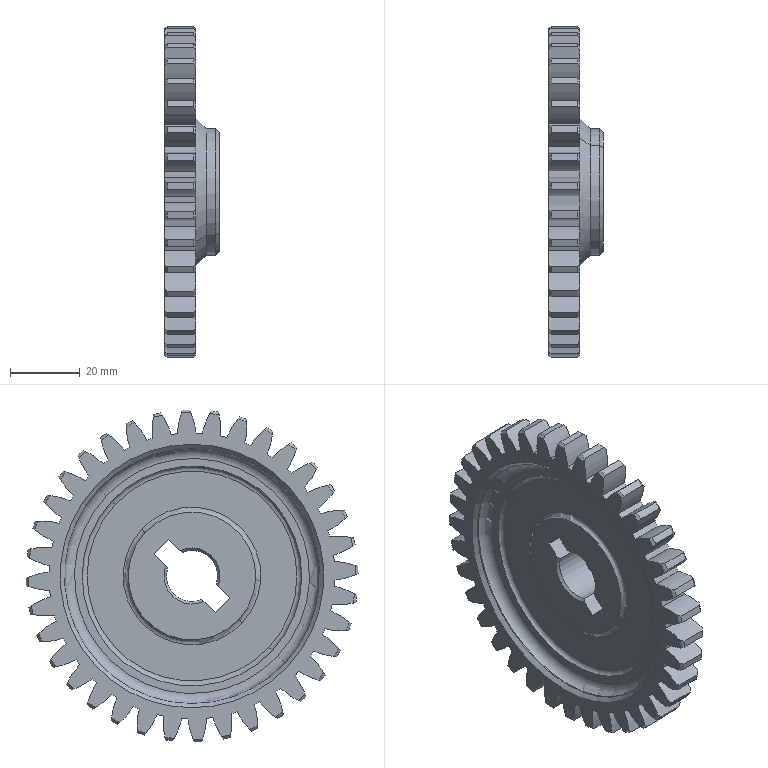Part | NX | 1 solid | 255 faces | box 15.665 x 95.15 x 95.15 mm | volume 40283 mm3 | cylinder 155 | cone 82 | plane 12 | torus 6 | commonest cylinder face diameters 43.92 x76 81.984 x37 95.16 x36 14.64 x2 36.454 x2 73.2 x2